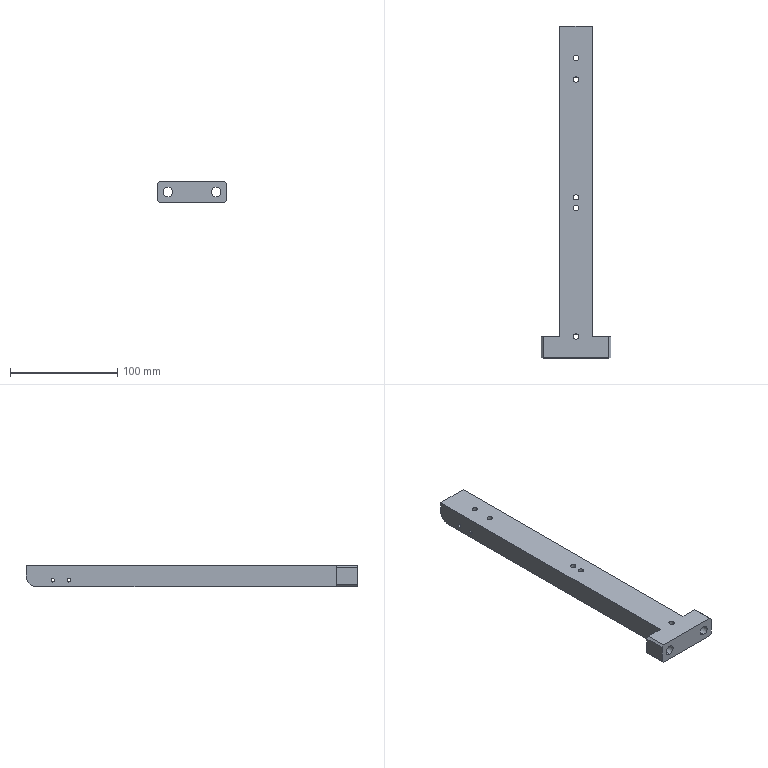Part | SolidWorks | features HoleWzd 3, Chamfer 1, Extrusion 1, Fillet 1 | 1 solid | 33 faces | box 65 x 310 x 20 mm | volume 194175 mm3 | cylinder 19 | plane 14 | commonest cylinder face diameters 5 x10 3.3 x4 9 x4 20 x1
STEP:
#1=CARTESIAN_POINT('',(15.,285.,4.35));
#2=VERTEX_POINT('',#1);
#3=CARTESIAN_POINT('',(15.,285.,7.65));
#4=VERTEX_POINT('',#3);
#5=CARTESIAN_POINT('',(15.,285.,6.));
#6=DIRECTION('',(-1.,0.,0.));
#7=DIRECTION('',(0.,-1.,0.));
#8=AXIS2_PLACEMENT_3D('',#5,#6,#7);
#9=CIRCLE('',#8,1.65);
#10=EDGE_CURVE('',#2,#4,#9,.T.);
#11=ORIENTED_EDGE('',*,*,#10,.F.);
#12=CARTESIAN_POINT('',(-15.,285.,4.35));
#13=VERTEX_POINT('',#12);
#14=CARTESIAN_POINT('',(-15.,285.,4.35));
#15=DIRECTION('',(-1.,0.,0.));
#16=VECTOR('',#15,1000.);
#17=LINE('',#14,#16);
#18=EDGE_CURVE('',#2,#13,#17,.T.);
#19=ORIENTED_EDGE('',*,*,#18,.T.);
#20=CARTESIAN_POINT('',(-15.,285.,7.65));
#21=VERTEX_POINT('',#20);
#22=CARTESIAN_POINT('',(-15.,285.,6.));
#23=DIRECTION('',(-1.,0.,0.));
#24=DIRECTION('',(0.,0.,1.));
#25=AXIS2_PLACEMENT_3D('',#22,#23,#24);
#26=CIRCLE('',#25,1.65);
#27=EDGE_CURVE('',#13,#21,#26,.T.);
#28=ORIENTED_EDGE('',*,*,#27,.T.);
#29=CARTESIAN_POINT('',(-15.,285.,7.65));
#30=DIRECTION('',(-1.,0.,0.));
#31=VECTOR('',#30,1000.);
#32=LINE('',#29,#31);
#33=EDGE_CURVE('',#4,#21,#32,.T.);
#34=ORIENTED_EDGE('',*,*,#33,.F.);
#35=EDGE_LOOP('',(#11,#19,#28,#34));
#36=FACE_OUTER_BOUND('',#35,.T.);
#37=CARTESIAN_POINT('',(-15.,285.,6.));
#38=DIRECTION('',(-1.,0.,0.));
#39=DIRECTION('',(0.,0.,1.));
#40=AXIS2_PLACEMENT_3D('',#37,#38,#39);
#41=CYLINDRICAL_SURFACE('',#40,1.65);
#42=ADVANCED_FACE('',(#36),#41,.F.);
#43=CARTESIAN_POINT('',(15.,270.,4.35));
#44=VERTEX_POINT('',#43);
#45=CARTESIAN_POINT('',(15.,270.,7.65));
#46=VERTEX_POINT('',#45);
#47=CARTESIAN_POINT('',(15.,270.,6.));
#48=DIRECTION('',(-1.,0.,0.));
#49=DIRECTION('',(0.,-1.,0.));
#50=AXIS2_PLACEMENT_3D('',#47,#48,#49);
#51=CIRCLE('',#50,1.65);
#52=EDGE_CURVE('',#44,#46,#51,.T.);
#53=ORIENTED_EDGE('',*,*,#52,.F.);
#54=CARTESIAN_POINT('',(-15.,270.,4.35));
#55=VERTEX_POINT('',#54);
#56=CARTESIAN_POINT('',(-15.,270.,4.35));
#57=DIRECTION('',(-1.,0.,0.));
#58=VECTOR('',#57,1000.);
#59=LINE('',#56,#58);
#60=EDGE_CURVE('',#44,#55,#59,.T.);
#61=ORIENTED_EDGE('',*,*,#60,.T.);
#62=CARTESIAN_POINT('',(-15.,270.,7.65));
#63=VERTEX_POINT('',#62);
#64=CARTESIAN_POINT('',(-15.,270.,6.));
#65=DIRECTION('',(-1.,0.,0.));
#66=DIRECTION('',(0.,0.,1.));
#67=AXIS2_PLACEMENT_3D('',#64,#65,#66);
#68=CIRCLE('',#67,1.65);
#69=EDGE_CURVE('',#55,#63,#68,.T.);
#70=ORIENTED_EDGE('',*,*,#69,.T.);
#71=CARTESIAN_POINT('',(-15.,270.,7.65));
#72=DIRECTION('',(-1.,0.,0.));
#73=VECTOR('',#72,1000.);
#74=LINE('',#71,#73);
#75=EDGE_CURVE('',#46,#63,#74,.T.);
#76=ORIENTED_EDGE('',*,*,#75,.F.);
#77=EDGE_LOOP('',(#53,#61,#70,#76));
#78=FACE_OUTER_BOUND('',#77,.T.);
#79=CARTESIAN_POINT('',(-15.,270.,6.));
#80=DIRECTION('',(-1.,0.,0.));
#81=DIRECTION('',(0.,0.,1.));
#82=AXIS2_PLACEMENT_3D('',#79,#80,#81);
#83=CYLINDRICAL_SURFACE('',#82,1.65);
#84=ADVANCED_FACE('',(#78),#83,.F.);
#85=CARTESIAN_POINT('',(-2.5,280.,0.));
#86=VERTEX_POINT('',#85);
#87=CARTESIAN_POINT('',(2.5,280.,0.));
#88=VERTEX_POINT('',#87);
#89=CARTESIAN_POINT('',(0.,280.,0.));
#90=DIRECTION('',(0.,0.,1.));
#91=DIRECTION('',(1.,0.,0.));
#92=AXIS2_PLACEMENT_3D('',#89,#90,#91);
#93=CIRCLE('',#92,2.5);
#94=EDGE_CURVE('',#86,#88,#93,.T.);
#95=ORIENTED_EDGE('',*,*,#94,.F.);
#96=CARTESIAN_POINT('',(-2.5,280.,20.));
#97=VERTEX_POINT('',#96);
#98=CARTESIAN_POINT('',(-2.5,280.,20.));
#99=DIRECTION('',(0.,0.,1.));
#100=VECTOR('',#99,1000.);
#101=LINE('',#98,#100);
#102=EDGE_CURVE('',#86,#97,#101,.T.);
#103=ORIENTED_EDGE('',*,*,#102,.T.);
#104=CARTESIAN_POINT('',(2.5,280.,20.));
#105=VERTEX_POINT('',#104);
#106=CARTESIAN_POINT('',(0.,280.,20.));
#107=DIRECTION('',(0.,0.,1.));
#108=DIRECTION('',(1.,0.,0.));
#109=AXIS2_PLACEMENT_3D('',#106,#107,#108);
#110=CIRCLE('',#109,2.5);
#111=EDGE_CURVE('',#97,#105,#110,.T.);
#112=ORIENTED_EDGE('',*,*,#111,.T.);
#113=CARTESIAN_POINT('',(2.5,280.,20.));
#114=DIRECTION('',(0.,0.,1.));
#115=VECTOR('',#114,1000.);
#116=LINE('',#113,#115);
#117=EDGE_CURVE('',#88,#105,#116,.T.);
#118=ORIENTED_EDGE('',*,*,#117,.F.);
#119=EDGE_LOOP('',(#95,#103,#112,#118));
#120=FACE_OUTER_BOUND('',#119,.T.);
#121=CARTESIAN_POINT('',(0.,280.,20.));
#122=DIRECTION('',(0.,0.,1.));
#123=DIRECTION('',(1.,0.,0.));
#124=AXIS2_PLACEMENT_3D('',#121,#122,#123);
#125=CYLINDRICAL_SURFACE('',#124,2.5);
#126=ADVANCED_FACE('',(#120),#125,.F.);
#127=CARTESIAN_POINT('',(-2.5,150.,0.));
#128=VERTEX_POINT('',#127);
#129=CARTESIAN_POINT('',(2.5,150.,0.));
#130=VERTEX_POINT('',#129);
#131=CARTESIAN_POINT('',(0.,150.,0.));
#132=DIRECTION('',(0.,0.,1.));
#133=DIRECTION('',(1.,0.,0.));
#134=AXIS2_PLACEMENT_3D('',#131,#132,#133);
#135=CIRCLE('',#134,2.5);
#136=EDGE_CURVE('',#128,#130,#135,.T.);
#137=ORIENTED_EDGE('',*,*,#136,.F.);
#138=CARTESIAN_POINT('',(-2.5,150.,20.));
#139=VERTEX_POINT('',#138);
#140=CARTESIAN_POINT('',(-2.5,150.,20.));
#141=DIRECTION('',(0.,0.,1.));
#142=VECTOR('',#141,1000.);
#143=LINE('',#140,#142);
#144=EDGE_CURVE('',#128,#139,#143,.T.);
#145=ORIENTED_EDGE('',*,*,#144,.T.);
#146=CARTESIAN_POINT('',(2.5,150.,20.));
#147=VERTEX_POINT('',#146);
#148=CARTESIAN_POINT('',(0.,150.,20.));
#149=DIRECTION('',(0.,0.,1.));
#150=DIRECTION('',(1.,0.,0.));
#151=AXIS2_PLACEMENT_3D('',#148,#149,#150);
#152=CIRCLE('',#151,2.5);
#153=EDGE_CURVE('',#139,#147,#152,.T.);
#154=ORIENTED_EDGE('',*,*,#153,.T.);
#155=CARTESIAN_POINT('',(2.5,150.,20.));
#156=DIRECTION('',(0.,0.,1.));
#157=VECTOR('',#156,1000.);
#158=LINE('',#155,#157);
#159=EDGE_CURVE('',#130,#147,#158,.T.);
#160=ORIENTED_EDGE('',*,*,#159,.F.);
#161=EDGE_LOOP('',(#137,#145,#154,#160));
#162=FACE_OUTER_BOUND('',#161,.T.);
#163=CARTESIAN_POINT('',(0.,150.,20.));
#164=DIRECTION('',(0.,0.,1.));
#165=DIRECTION('',(1.,0.,0.));
#166=AXIS2_PLACEMENT_3D('',#163,#164,#165);
#167=CYLINDRICAL_SURFACE('',#166,2.5);
#168=ADVANCED_FACE('',(#162),#167,.F.);
#169=CARTESIAN_POINT('',(-2.5,20.,0.));
#170=VERTEX_POINT('',#169);
#171=CARTESIAN_POINT('',(2.5,20.,0.));
#172=VERTEX_POINT('',#171);
#173=CARTESIAN_POINT('',(0.,20.,0.));
#174=DIRECTION('',(0.,0.,1.));
#175=DIRECTION('',(1.,0.,0.));
#176=AXIS2_PLACEMENT_3D('',#173,#174,#175);
#177=CIRCLE('',#176,2.5);
#178=EDGE_CURVE('',#170,#172,#177,.T.);
#179=ORIENTED_EDGE('',*,*,#178,.F.);
#180=CARTESIAN_POINT('',(-2.5,20.,20.));
#181=VERTEX_POINT('',#180);
#182=CARTESIAN_POINT('',(-2.5,20.,20.));
#183=DIRECTION('',(0.,0.,1.));
#184=VECTOR('',#183,1000.);
#185=LINE('',#182,#184);
#186=EDGE_CURVE('',#170,#181,#185,.T.);
#187=ORIENTED_EDGE('',*,*,#186,.T.);
#188=CARTESIAN_POINT('',(2.5,20.,20.));
#189=VERTEX_POINT('',#188);
#190=CARTESIAN_POINT('',(0.,20.,20.));
#191=DIRECTION('',(0.,0.,1.));
#192=DIRECTION('',(1.,0.,0.));
#193=AXIS2_PLACEMENT_3D('',#190,#191,#192);
#194=CIRCLE('',#193,2.5);
#195=EDGE_CURVE('',#181,#189,#194,.T.);
#196=ORIENTED_EDGE('',*,*,#195,.T.);
#197=CARTESIAN_POINT('',(2.5,20.,20.));
#198=DIRECTION('',(0.,0.,1.));
#199=VECTOR('',#198,1000.);
#200=LINE('',#197,#199);
#201=EDGE_CURVE('',#172,#189,#200,.T.);
#202=ORIENTED_EDGE('',*,*,#201,.F.);
#203=EDGE_LOOP('',(#179,#187,#196,#202));
#204=FACE_OUTER_BOUND('',#203,.T.);
#205=CARTESIAN_POINT('',(0.,20.,20.));
#206=DIRECTION('',(0.,0.,1.));
#207=DIRECTION('',(1.,0.,0.));
#208=AXIS2_PLACEMENT_3D('',#205,#206,#207);
#209=CYLINDRICAL_SURFACE('',#208,2.5);
#210=ADVANCED_FACE('',(#204),#209,.F.);
#211=CARTESIAN_POINT('',(-2.5,260.,0.));
#212=VERTEX_POINT('',#211);
#213=CARTESIAN_POINT('',(2.5,260.,0.));
#214=VERTEX_POINT('',#213);
#215=CARTESIAN_POINT('',(0.,260.,0.));
#216=DIRECTION('',(0.,0.,1.));
#217=DIRECTION('',(1.,0.,0.));
#218=AXIS2_PLACEMENT_3D('',#215,#216,#217);
#219=CIRCLE('',#218,2.5);
#220=EDGE_CURVE('',#212,#214,#219,.T.);
#221=ORIENTED_EDGE('',*,*,#220,.F.);
#222=CARTESIAN_POINT('',(-2.5,260.,20.));
#223=VERTEX_POINT('',#222);
#224=CARTESIAN_POINT('',(-2.5,260.,20.));
#225=DIRECTION('',(0.,0.,1.));
#226=VECTOR('',#225,1000.);
#227=LINE('',#224,#226);
#228=EDGE_CURVE('',#212,#223,#227,.T.);
#229=ORIENTED_EDGE('',*,*,#228,.T.);
#230=CARTESIAN_POINT('',(2.5,260.,20.));
#231=VERTEX_POINT('',#230);
#232=CARTESIAN_POINT('',(0.,260.,20.));
#233=DIRECTION('',(0.,0.,1.));
#234=DIRECTION('',(1.,0.,0.));
#235=AXIS2_PLACEMENT_3D('',#232,#233,#234);
#236=CIRCLE('',#235,2.5);
#237=EDGE_CURVE('',#223,#231,#236,.T.);
#238=ORIENTED_EDGE('',*,*,#237,.T.);
#239=CARTESIAN_POINT('',(2.5,260.,20.));
#240=DIRECTION('',(0.,0.,1.));
#241=VECTOR('',#240,1000.);
#242=LINE('',#239,#241);
#243=EDGE_CURVE('',#214,#231,#242,.T.);
#244=ORIENTED_EDGE('',*,*,#243,.F.);
#245=EDGE_LOOP('',(#221,#229,#238,#244));
#246=FACE_OUTER_BOUND('',#245,.T.);
#247=CARTESIAN_POINT('',(0.,260.,20.));
#248=DIRECTION('',(0.,0.,1.));
#249=DIRECTION('',(1.,0.,0.));
#250=AXIS2_PLACEMENT_3D('',#247,#248,#249);
#251=CYLINDRICAL_SURFACE('',#250,2.5);
#252=ADVANCED_FACE('',(#246),#251,.F.);
#253=CARTESIAN_POINT('',(-2.5,140.,0.));
#254=VERTEX_POINT('',#253);
#255=CARTESIAN_POINT('',(2.5,140.,0.));
#256=VERTEX_POINT('',#255);
#257=CARTESIAN_POINT('',(0.,140.,0.));
#258=DIRECTION('',(0.,0.,1.));
#259=DIRECTION('',(1.,0.,0.));
#260=AXIS2_PLACEMENT_3D('',#257,#258,#259);
#261=CIRCLE('',#260,2.5);
#262=EDGE_CURVE('',#254,#256,#261,.T.);
#263=ORIENTED_EDGE('',*,*,#262,.F.);
#264=CARTESIAN_POINT('',(-2.5,140.,20.));
#265=VERTEX_POINT('',#264);
#266=CARTESIAN_POINT('',(-2.5,140.,20.));
#267=DIRECTION('',(0.,0.,1.));
#268=VECTOR('',#267,1000.);
#269=LINE('',#266,#268);
#270=EDGE_CURVE('',#254,#265,#269,.T.);
#271=ORIENTED_EDGE('',*,*,#270,.T.);
#272=CARTESIAN_POINT('',(2.5,140.,20.));
#273=VERTEX_POINT('',#272);
#274=CARTESIAN_POINT('',(0.,140.,20.));
#275=DIRECTION('',(0.,0.,1.));
#276=DIRECTION('',(1.,0.,0.));
#277=AXIS2_PLACEMENT_3D('',#274,#275,#276);
#278=CIRCLE('',#277,2.5);
#279=EDGE_CURVE('',#265,#273,#278,.T.);
#280=ORIENTED_EDGE('',*,*,#279,.T.);
#281=CARTESIAN_POINT('',(2.5,140.,20.));
#282=DIRECTION('',(0.,0.,1.));
#283=VECTOR('',#282,1000.);
#284=LINE('',#281,#283);
#285=EDGE_CURVE('',#256,#273,#284,.T.);
#286=ORIENTED_EDGE('',*,*,#285,.F.);
#287=EDGE_LOOP('',(#263,#271,#280,#286));
#288=FACE_OUTER_BOUND('',#287,.T.);
#289=CARTESIAN_POINT('',(0.,140.,20.));
#290=DIRECTION('',(0.,0.,1.));
#291=DIRECTION('',(1.,0.,0.));
#292=AXIS2_PLACEMENT_3D('',#289,#290,#291);
#293=CYLINDRICAL_SURFACE('',#292,2.5);
#294=ADVANCED_FACE('',(#288),#293,.F.);
#295=CARTESIAN_POINT('',(22.5,0.,5.5));
#296=VERTEX_POINT('',#295);
#297=CARTESIAN_POINT('',(22.5,0.,14.5));
#298=VERTEX_POINT('',#297);
#299=CARTESIAN_POINT('',(22.5,0.,10.));
#300=DIRECTION('',(0.,1.,0.));
#301=DIRECTION('',(0.,0.,1.));
#302=AXIS2_PLACEMENT_3D('',#299,#300,#301);
#303=CIRCLE('',#302,4.5);
#304=EDGE_CURVE('',#296,#298,#303,.T.);
#305=ORIENTED_EDGE('',*,*,#304,.F.);
#306=CARTESIAN_POINT('',(22.5,20.,5.5));
#307=VERTEX_POINT('',#306);
#308=CARTESIAN_POINT('',(22.5,20.,5.5));
#309=DIRECTION('',(0.,1.,0.));
#310=VECTOR('',#309,1000.);
#311=LINE('',#308,#310);
#312=EDGE_CURVE('',#296,#307,#311,.T.);
#313=ORIENTED_EDGE('',*,*,#312,.T.);
#314=CARTESIAN_POINT('',(22.5,20.,14.5));
#315=VERTEX_POINT('',#314);
#316=CARTESIAN_POINT('',(22.5,20.,10.));
#317=DIRECTION('',(0.,1.,0.));
#318=DIRECTION('',(0.,0.,1.));
#319=AXIS2_PLACEMENT_3D('',#316,#317,#318);
#320=CIRCLE('',#319,4.5);
#321=EDGE_CURVE('',#307,#315,#320,.T.);
#322=ORIENTED_EDGE('',*,*,#321,.T.);
#323=CARTESIAN_POINT('',(22.5,20.,14.5));
#324=DIRECTION('',(0.,1.,0.));
#325=VECTOR('',#324,1000.);
#326=LINE('',#323,#325);
#327=EDGE_CURVE('',#298,#315,#326,.T.);
#328=ORIENTED_EDGE('',*,*,#327,.F.);
#329=EDGE_LOOP('',(#305,#313,#322,#328));
#330=FACE_OUTER_BOUND('',#329,.T.);
#331=CARTESIAN_POINT('',(22.5,20.,10.));
#332=DIRECTION('',(0.,1.,0.));
#333=DIRECTION('',(0.,0.,1.));
#334=AXIS2_PLACEMENT_3D('',#331,#332,#333);
#335=CYLINDRICAL_SURFACE('',#334,4.5);
#336=ADVANCED_FACE('',(#330),#335,.F.);
#337=CARTESIAN_POINT('',(-22.5,0.,5.5));
#338=VERTEX_POINT('',#337);
#339=CARTESIAN_POINT('',(-22.5,0.,14.5));
#340=VERTEX_POINT('',#339);
#341=CARTESIAN_POINT('',(-22.5,0.,10.));
#342=DIRECTION('',(0.,1.,0.));
#343=DIRECTION('',(0.,0.,1.));
#344=AXIS2_PLACEMENT_3D('',#341,#342,#343);
#345=CIRCLE('',#344,4.5);
#346=EDGE_CURVE('',#338,#340,#345,.T.);
#347=ORIENTED_EDGE('',*,*,#346,.F.);
#348=CARTESIAN_POINT('',(-22.5,20.,5.5));
#349=VERTEX_POINT('',#348);
#350=CARTESIAN_POINT('',(-22.5,20.,5.5));
#351=DIRECTION('',(0.,1.,0.));
#352=VECTOR('',#351,1000.);
#353=LINE('',#350,#352);
#354=EDGE_CURVE('',#338,#349,#353,.T.);
#355=ORIENTED_EDGE('',*,*,#354,.T.);
#356=CARTESIAN_POINT('',(-22.5,20.,14.5));
#357=VERTEX_POINT('',#356);
#358=CARTESIAN_POINT('',(-22.5,20.,10.));
#359=DIRECTION('',(0.,1.,0.));
#360=DIRECTION('',(0.,0.,1.));
#361=AXIS2_PLACEMENT_3D('',#358,#359,#360);
#362=CIRCLE('',#361,4.5);
#363=EDGE_CURVE('',#349,#357,#362,.T.);
#364=ORIENTED_EDGE('',*,*,#363,.T.);
#365=CARTESIAN_POINT('',(-22.5,20.,14.5));
#366=DIRECTION('',(0.,1.,0.));
#367=VECTOR('',#366,1000.);
#368=LINE('',#365,#367);
#369=EDGE_CURVE('',#340,#357,#368,.T.);
#370=ORIENTED_EDGE('',*,*,#369,.F.);
#371=EDGE_LOOP('',(#347,#355,#364,#370));
#372=FACE_OUTER_BOUND('',#371,.T.);
#373=CARTESIAN_POINT('',(-22.5,20.,10.));
#374=DIRECTION('',(0.,1.,0.));
#375=DIRECTION('',(0.,0.,1.));
#376=AXIS2_PLACEMENT_3D('',#373,#374,#375);
#377=CYLINDRICAL_SURFACE('',#376,4.5);
#378=ADVANCED_FACE('',(#372),#377,.F.);
#379=CARTESIAN_POINT('',(-15.,285.,6.));
#380=DIRECTION('',(-1.,0.,0.));
#381=DIRECTION('',(0.,0.,1.));
#382=AXIS2_PLACEMENT_3D('',#379,#380,#381);
#383=CIRCLE('',#382,1.65);
#384=EDGE_CURVE('',#21,#13,#383,.T.);
#385=ORIENTED_EDGE('',*,*,#384,.F.);
#386=ORIENTED_EDGE('',*,*,#27,.F.);
#387=EDGE_LOOP('',(#385,#386));
#388=FACE_BOUND('',#387,.T.);
#389=CARTESIAN_POINT('',(-15.,270.,6.));
#390=DIRECTION('',(-1.,0.,0.));
#391=DIRECTION('',(0.,0.,1.));
#392=AXIS2_PLACEMENT_3D('',#389,#390,#391);
#393=CIRCLE('',#392,1.65);
#394=EDGE_CURVE('',#63,#55,#393,.T.);
#395=ORIENTED_EDGE('',*,*,#394,.F.);
#396=ORIENTED_EDGE('',*,*,#69,.F.);
#397=EDGE_LOOP('',(#395,#396));
#398=FACE_BOUND('',#397,.T.);
#399=CARTESIAN_POINT('',(-15.,310.,20.));
#400=VERTEX_POINT('',#399);
#401=CARTESIAN_POINT('',(-15.,310.,10.));
#402=VERTEX_POINT('',#401);
#403=CARTESIAN_POINT('',(-15.,310.,20.));
#404=DIRECTION('',(0.,0.,-1.));
#405=VECTOR('',#404,1000.);
#406=LINE('',#403,#405);
#407=EDGE_CURVE('',#400,#402,#406,.T.);
#408=ORIENTED_EDGE('',*,*,#407,.T.);
#409=CARTESIAN_POINT('',(-15.,300.,0.));
#410=VERTEX_POINT('',#409);
#411=CARTESIAN_POINT('',(-15.,300.,10.));
#412=DIRECTION('',(-1.,0.,0.));
#413=DIRECTION('',(0.,1.,0.));
#414=AXIS2_PLACEMENT_3D('',#411,#412,#413);
#415=CIRCLE('',#414,10.);
#416=EDGE_CURVE('',#402,#410,#415,.T.);
#417=ORIENTED_EDGE('',*,*,#416,.T.);
#418=CARTESIAN_POINT('',(-15.,20.,0.));
#419=VERTEX_POINT('',#418);
#420=CARTESIAN_POINT('',(-15.,310.,0.));
#421=DIRECTION('',(0.,-1.,0.));
#422=VECTOR('',#421,1000.);
#423=LINE('',#420,#422);
#424=EDGE_CURVE('',#410,#419,#423,.T.);
#425=ORIENTED_EDGE('',*,*,#424,.T.);
#426=CARTESIAN_POINT('',(-15.,20.,20.));
#427=VERTEX_POINT('',#426);
#428=CARTESIAN_POINT('',(-15.,20.,20.));
#429=DIRECTION('',(0.,0.,-1.));
#430=VECTOR('',#429,1000.);
#431=LINE('',#428,#430);
#432=EDGE_CURVE('',#427,#419,#431,.T.);
#433=ORIENTED_EDGE('',*,*,#432,.F.);
#434=CARTESIAN_POINT('',(-15.,310.,20.));
#435=DIRECTION('',(0.,-1.,0.));
#436=VECTOR('',#435,1000.);
#437=LINE('',#434,#436);
#438=EDGE_CURVE('',#400,#427,#437,.T.);
#439=ORIENTED_EDGE('',*,*,#438,.F.);
#440=EDGE_LOOP('',(#408,#417,#425,#433,#439));
#441=FACE_OUTER_BOUND('',#440,.T.);
#442=CARTESIAN_POINT('',(-15.,310.,20.));
#443=DIRECTION('',(1.,0.,0.));
#444=DIRECTION('',(0.,1.,0.));
#445=AXIS2_PLACEMENT_3D('',#442,#443,#444);
#446=PLANE('',#445);
#447=ADVANCED_FACE('',(#388,#398,#441),#446,.F.);
#448=CARTESIAN_POINT('',(-22.5,20.,10.));
#449=DIRECTION('',(0.,1.,0.));
#450=DIRECTION('',(0.,0.,1.));
#451=AXIS2_PLACEMENT_3D('',#448,#449,#450);
#452=CIRCLE('',#451,4.5);
#453=EDGE_CURVE('',#357,#349,#452,.T.);
#454=ORIENTED_EDGE('',*,*,#453,.F.);
#455=ORIENTED_EDGE('',*,*,#363,.F.);
#456=EDGE_LOOP('',(#454,#455));
#457=FACE_BOUND('',#456,.T.);
#458=CARTESIAN_POINT('',(-32.5,20.,18.));
#459=VERTEX_POINT('',#458);
#460=CARTESIAN_POINT('',(-32.5,20.,2.));
#461=VERTEX_POINT('',#460);
#462=CARTESIAN_POINT('',(-32.5,20.,20.));
#463=DIRECTION('',(0.,0.,-1.));
#464=VECTOR('',#463,1000.);
#465=LINE('',#462,#464);
#466=EDGE_CURVE('',#459,#461,#465,.T.);
#467=ORIENTED_EDGE('',*,*,#466,.F.);
#468=CARTESIAN_POINT('',(-30.5,20.,20.));
#469=VERTEX_POINT('',#468);
#470=CARTESIAN_POINT('',(-30.5,20.,20.));
#471=DIRECTION('',(0.7071,0.,0.7071));
#472=VECTOR('',#471,1000.);
#473=LINE('',#470,#472);
#474=EDGE_CURVE('',#459,#469,#473,.T.);
#475=ORIENTED_EDGE('',*,*,#474,.T.);
#476=CARTESIAN_POINT('',(-15.,20.,20.));
#477=DIRECTION('',(-1.,0.,0.));
#478=VECTOR('',#477,1000.);
#479=LINE('',#476,#478);
#480=EDGE_CURVE('',#427,#469,#479,.T.);
#481=ORIENTED_EDGE('',*,*,#480,.F.);
#482=ORIENTED_EDGE('',*,*,#432,.T.);
#483=CARTESIAN_POINT('',(-30.5,20.,0.));
#484=VERTEX_POINT('',#483);
#485=CARTESIAN_POINT('',(-15.,20.,0.));
#486=DIRECTION('',(-1.,0.,0.));
#487=VECTOR('',#486,1000.);
#488=LINE('',#485,#487);
#489=EDGE_CURVE('',#419,#484,#488,.T.);
#490=ORIENTED_EDGE('',*,*,#489,.T.);
#491=CARTESIAN_POINT('',(-32.5,20.,2.));
#492=DIRECTION('',(-0.7071,0.,0.7071));
#493=VECTOR('',#492,1000.);
#494=LINE('',#491,#493);
#495=EDGE_CURVE('',#484,#461,#494,.T.);
#496=ORIENTED_EDGE('',*,*,#495,.T.);
#497=EDGE_LOOP('',(#467,#475,#481,#482,#490,#496));
#498=FACE_OUTER_BOUND('',#497,.T.);
#499=CARTESIAN_POINT('',(-15.,20.,20.));
#500=DIRECTION('',(0.,-1.,0.));
#501=DIRECTION('',(1.,0.,0.));
#502=AXIS2_PLACEMENT_3D('',#499,#500,#501);
#503=PLANE('',#502);
#504=ADVANCED_FACE('',(#457,#498),#503,.F.);
#505=CARTESIAN_POINT('',(-32.5,0.,18.));
#506=VERTEX_POINT('',#505);
#507=CARTESIAN_POINT('',(-32.5,0.,2.));
#508=VERTEX_POINT('',#507);
#509=CARTESIAN_POINT('',(-32.5,0.,20.));
#510=DIRECTION('',(0.,0.,-1.));
#511=VECTOR('',#510,1000.);
#512=LINE('',#509,#511);
#513=EDGE_CURVE('',#506,#508,#512,.T.);
#514=ORIENTED_EDGE('',*,*,#513,.F.);
#515=CARTESIAN_POINT('',(-32.5,20.,18.));
#516=DIRECTION('',(0.,1.,0.));
#517=VECTOR('',#516,1000.);
#518=LINE('',#515,#517);
#519=EDGE_CURVE('',#506,#459,#518,.T.);
#520=ORIENTED_EDGE('',*,*,#519,.T.);
#521=ORIENTED_EDGE('',*,*,#466,.T.);
#522=CARTESIAN_POINT('',(-32.5,0.,2.));
#523=DIRECTION('',(0.,-1.,0.));
#524=VECTOR('',#523,1000.);
#525=LINE('',#522,#524);
#526=EDGE_CURVE('',#461,#508,#525,.T.);
#527=ORIENTED_EDGE('',*,*,#526,.T.);
#528=EDGE_LOOP('',(#514,#520,#521,#527));
#529=FACE_OUTER_BOUND('',#528,.T.);
#530=CARTESIAN_POINT('',(-32.5,20.,20.));
#531=DIRECTION('',(1.,0.,0.));
#532=DIRECTION('',(0.,1.,0.));
#533=AXIS2_PLACEMENT_3D('',#530,#531,#532);
#534=PLANE('',#533);
#535=ADVANCED_FACE('',(#529),#534,.F.);
#536=CARTESIAN_POINT('',(22.5,0.,10.));
#537=DIRECTION('',(0.,1.,0.));
#538=DIRECTION('',(0.,0.,1.));
#539=AXIS2_PLACEMENT_3D('',#536,#537,#538);
#540=CIRCLE('',#539,4.5);
#541=EDGE_CURVE('',#298,#296,#540,.T.);
#542=ORIENTED_EDGE('',*,*,#541,.T.);
#543=ORIENTED_EDGE('',*,*,#304,.T.);
#544=EDGE_LOOP('',(#542,#543));
#545=FACE_BOUND('',#544,.T.);
#546=CARTESIAN_POINT('',(-22.5,0.,10.));
#547=DIRECTION('',(0.,1.,0.));
#548=DIRECTION('',(0.,0.,1.));
#549=AXIS2_PLACEMENT_3D('',#546,#547,#548);
#550=CIRCLE('',#549,4.5);
#551=EDGE_CURVE('',#340,#338,#550,.T.);
#552=ORIENTED_EDGE('',*,*,#551,.T.);
#553=ORIENTED_EDGE('',*,*,#346,.T.);
#554=EDGE_LOOP('',(#552,#553));
#555=FACE_BOUND('',#554,.T.);
#556=CARTESIAN_POINT('',(32.5,0.,18.));
#557=VERTEX_POINT('',#556);
#558=CARTESIAN_POINT('',(32.5,0.,2.));
#559=VERTEX_POINT('',#558);
#560=CARTESIAN_POINT('',(32.5,0.,20.));
#561=DIRECTION('',(0.,0.,-1.));
#562=VECTOR('',#561,1000.);
#563=LINE('',#560,#562);
#564=EDGE_CURVE('',#557,#559,#563,.T.);
#565=ORIENTED_EDGE('',*,*,#564,.F.);
#566=CARTESIAN_POINT('',(30.5,0.,20.));
#567=VERTEX_POINT('',#566);
#568=CARTESIAN_POINT('',(30.5,0.,20.));
#569=DIRECTION('',(-0.7071,0.,0.7071));
#570=VECTOR('',#569,1000.);
#571=LINE('',#568,#570);
#572=EDGE_CURVE('',#557,#567,#571,.T.);
#573=ORIENTED_EDGE('',*,*,#572,.T.);
#574=CARTESIAN_POINT('',(-30.5,0.,20.));
#575=VERTEX_POINT('',#574);
#576=CARTESIAN_POINT('',(-32.5,0.,20.));
#577=DIRECTION('',(1.,0.,0.));
#578=VECTOR('',#577,1000.);
#579=LINE('',#576,#578);
#580=EDGE_CURVE('',#575,#567,#579,.T.);
#581=ORIENTED_EDGE('',*,*,#580,.F.);
#582=CARTESIAN_POINT('',(-30.5,0.,20.));
#583=DIRECTION('',(-0.7071,0.,-0.7071));
#584=VECTOR('',#583,1000.);
#585=LINE('',#582,#584);
#586=EDGE_CURVE('',#575,#506,#585,.T.);
#587=ORIENTED_EDGE('',*,*,#586,.T.);
#588=ORIENTED_EDGE('',*,*,#513,.T.);
#589=CARTESIAN_POINT('',(-30.5,0.,0.));
#590=VERTEX_POINT('',#589);
#591=CARTESIAN_POINT('',(-32.5,0.,2.));
#592=DIRECTION('',(0.7071,0.,-0.7071));
#593=VECTOR('',#592,1000.);
#594=LINE('',#591,#593);
#595=EDGE_CURVE('',#508,#590,#594,.T.);
#596=ORIENTED_EDGE('',*,*,#595,.T.);
#597=CARTESIAN_POINT('',(30.5,0.,0.));
#598=VERTEX_POINT('',#597);
#599=CARTESIAN_POINT('',(-32.5,0.,0.));
#600=DIRECTION('',(1.,0.,0.));
#601=VECTOR('',#600,1000.);
#602=LINE('',#599,#601);
#603=EDGE_CURVE('',#590,#598,#602,.T.);
#604=ORIENTED_EDGE('',*,*,#603,.T.);
#605=CARTESIAN_POINT('',(32.5,0.,2.));
#606=DIRECTION('',(0.7071,0.,0.7071));
#607=VECTOR('',#606,1000.);
#608=LINE('',#605,#607);
#609=EDGE_CURVE('',#598,#559,#608,.T.);
#610=ORIENTED_EDGE('',*,*,#609,.T.);
#611=EDGE_LOOP('',(#565,#573,#581,#587,#588,#596,#604,#610));
#612=FACE_OUTER_BOUND('',#611,.T.);
#613=CARTESIAN_POINT('',(-32.5,0.,20.));
#614=DIRECTION('',(0.,1.,0.));
#615=DIRECTION('',(0.,0.,1.));
#616=AXIS2_PLACEMENT_3D('',#613,#614,#615);
#617=PLANE('',#616);
#618=ADVANCED_FACE('',(#545,#555,#612),#617,.F.);
#619=CARTESIAN_POINT('',(32.5,20.,18.));
#620=VERTEX_POINT('',#619);
#621=CARTESIAN_POINT('',(32.5,20.,2.));
#622=VERTEX_POINT('',#621);
#623=CARTESIAN_POINT('',(32.5,20.,20.));
#624=DIRECTION('',(0.,0.,-1.));
#625=VECTOR('',#624,1000.);
#626=LINE('',#623,#625);
#627=EDGE_CURVE('',#620,#622,#626,.T.);
#628=ORIENTED_EDGE('',*,*,#627,.F.);
#629=CARTESIAN_POINT('',(32.5,20.,18.));
#630=DIRECTION('',(0.,-1.,0.));
#631=VECTOR('',#630,1000.);
#632=LINE('',#629,#631);
#633=EDGE_CURVE('',#620,#557,#632,.T.);
#634=ORIENTED_EDGE('',*,*,#633,.T.);
#635=ORIENTED_EDGE('',*,*,#564,.T.);
#636=CARTESIAN_POINT('',(32.5,20.,2.));
#637=DIRECTION('',(0.,1.,0.));
#638=VECTOR('',#637,1000.);
#639=LINE('',#636,#638);
#640=EDGE_CURVE('',#559,#622,#639,.T.);
#641=ORIENTED_EDGE('',*,*,#640,.T.);
#642=EDGE_LOOP('',(#628,#634,#635,#641));
#643=FACE_OUTER_BOUND('',#642,.T.);
#644=CARTESIAN_POINT('',(32.5,20.,20.));
#645=DIRECTION('',(-1.,0.,0.));
#646=DIRECTION('',(0.,-1.,0.));
#647=AXIS2_PLACEMENT_3D('',#644,#645,#646);
#648=PLANE('',#647);
#649=ADVANCED_FACE('',(#643),#648,.F.);
#650=CARTESIAN_POINT('',(22.5,20.,10.));
#651=DIRECTION('',(0.,1.,0.));
#652=DIRECTION('',(0.,0.,1.));
#653=AXIS2_PLACEMENT_3D('',#650,#651,#652);
#654=CIRCLE('',#653,4.5);
#655=EDGE_CURVE('',#315,#307,#654,.T.);
#656=ORIENTED_EDGE('',*,*,#655,.F.);
#657=ORIENTED_EDGE('',*,*,#321,.F.);
#658=EDGE_LOOP('',(#656,#657));
#659=FACE_BOUND('',#658,.T.);
#660=CARTESIAN_POINT('',(30.5,20.,20.));
#661=VERTEX_POINT('',#660);
#662=CARTESIAN_POINT('',(15.,20.,20.));
#663=VERTEX_POINT('',#662);
#664=CARTESIAN_POINT('',(15.,20.,20.));
#665=DIRECTION('',(-1.,0.,0.));
#666=VECTOR('',#665,1000.);
#667=LINE('',#664,#666);
#668=EDGE_CURVE('',#661,#663,#667,.T.);
#669=ORIENTED_EDGE('',*,*,#668,.F.);
#670=CARTESIAN_POINT('',(30.5,20.,20.));
#671=DIRECTION('',(0.7071,0.,-0.7071));
#672=VECTOR('',#671,1000.);
#673=LINE('',#670,#672);
#674=EDGE_CURVE('',#661,#620,#673,.T.);
#675=ORIENTED_EDGE('',*,*,#674,.T.);
#676=ORIENTED_EDGE('',*,*,#627,.T.);
#677=CARTESIAN_POINT('',(30.5,20.,0.));
#678=VERTEX_POINT('',#677);
#679=CARTESIAN_POINT('',(32.5,20.,2.));
#680=DIRECTION('',(-0.7071,0.,-0.7071));
#681=VECTOR('',#680,1000.);
#682=LINE('',#679,#681);
#683=EDGE_CURVE('',#622,#678,#682,.T.);
#684=ORIENTED_EDGE('',*,*,#683,.T.);
#685=CARTESIAN_POINT('',(15.,20.,0.));
#686=VERTEX_POINT('',#685);
#687=CARTESIAN_POINT('',(15.,20.,0.));
#688=DIRECTION('',(-1.,0.,0.));
#689=VECTOR('',#688,1000.);
#690=LINE('',#687,#689);
#691=EDGE_CURVE('',#678,#686,#690,.T.);
#692=ORIENTED_EDGE('',*,*,#691,.T.);
#693=CARTESIAN_POINT('',(15.,20.,20.));
#694=DIRECTION('',(0.,0.,-1.));
#695=VECTOR('',#694,1000.);
#696=LINE('',#693,#695);
#697=EDGE_CURVE('',#663,#686,#696,.T.);
#698=ORIENTED_EDGE('',*,*,#697,.F.);
#699=EDGE_LOOP('',(#669,#675,#676,#684,#692,#698));
#700=FACE_OUTER_BOUND('',#699,.T.);
#701=CARTESIAN_POINT('',(15.,20.,20.));
#702=DIRECTION('',(0.,-1.,0.));
#703=DIRECTION('',(1.,0.,0.));
#704=AXIS2_PLACEMENT_3D('',#701,#702,#703);
#705=PLANE('',#704);
#706=ADVANCED_FACE('',(#659,#700),#705,.F.);
#707=CARTESIAN_POINT('',(15.,285.,6.));
#708=DIRECTION('',(-1.,0.,0.));
#709=DIRECTION('',(0.,-1.,0.));
#710=AXIS2_PLACEMENT_3D('',#707,#708,#709);
#711=CIRCLE('',#710,1.65);
#712=EDGE_CURVE('',#4,#2,#711,.T.);
#713=ORIENTED_EDGE('',*,*,#712,.T.);
#714=ORIENTED_EDGE('',*,*,#10,.T.);
#715=EDGE_LOOP('',(#713,#714));
#716=FACE_BOUND('',#715,.T.);
#717=CARTESIAN_POINT('',(15.,270.,6.));
#718=DIRECTION('',(-1.,0.,0.));
#719=DIRECTION('',(0.,-1.,0.));
#720=AXIS2_PLACEMENT_3D('',#717,#718,#719);
#721=CIRCLE('',#720,1.65);
#722=EDGE_CURVE('',#46,#44,#721,.T.);
#723=ORIENTED_EDGE('',*,*,#722,.T.);
#724=ORIENTED_EDGE('',*,*,#52,.T.);
#725=EDGE_LOOP('',(#723,#724));
#726=FACE_BOUND('',#725,.T.);
#727=CARTESIAN_POINT('',(15.,300.,0.));
#728=VERTEX_POINT('',#727);
#729=CARTESIAN_POINT('',(15.,310.,0.));
#730=DIRECTION('',(0.,1.,0.));
#731=VECTOR('',#730,1000.);
#732=LINE('',#729,#731);
#733=EDGE_CURVE('',#686,#728,#732,.T.);
#734=ORIENTED_EDGE('',*,*,#733,.T.);
#735=CARTESIAN_POINT('',(15.,310.,10.));
#736=VERTEX_POINT('',#735);
#737=CARTESIAN_POINT('',(15.,300.,10.));
#738=DIRECTION('',(1.,0.,0.));
#739=DIRECTION('',(0.,-1.,0.));
#740=AXIS2_PLACEMENT_3D('',#737,#738,#739);
#741=CIRCLE('',#740,10.);
#742=EDGE_CURVE('',#728,#736,#741,.T.);
#743=ORIENTED_EDGE('',*,*,#742,.T.);
#744=CARTESIAN_POINT('',(15.,310.,20.));
#745=VERTEX_POINT('',#744);
#746=CARTESIAN_POINT('',(15.,310.,20.));
#747=DIRECTION('',(0.,0.,-1.));
#748=VECTOR('',#747,1000.);
#749=LINE('',#746,#748);
#750=EDGE_CURVE('',#745,#736,#749,.T.);
#751=ORIENTED_EDGE('',*,*,#750,.F.);
#752=CARTESIAN_POINT('',(15.,310.,20.));
#753=DIRECTION('',(0.,1.,0.));
#754=VECTOR('',#753,1000.);
#755=LINE('',#752,#754);
#756=EDGE_CURVE('',#663,#745,#755,.T.);
#757=ORIENTED_EDGE('',*,*,#756,.F.);
#758=ORIENTED_EDGE('',*,*,#697,.T.);
#759=EDGE_LOOP('',(#734,#743,#751,#757,#758));
#760=FACE_OUTER_BOUND('',#759,.T.);
#761=CARTESIAN_POINT('',(15.,310.,20.));
#762=DIRECTION('',(-1.,0.,0.));
#763=DIRECTION('',(0.,-1.,0.));
#764=AXIS2_PLACEMENT_3D('',#761,#762,#763);
#765=PLANE('',#764);
#766=ADVANCED_FACE('',(#716,#726,#760),#765,.F.);
#767=ORIENTED_EDGE('',*,*,#750,.T.);
#768=CARTESIAN_POINT('',(-15.,310.,10.));
#769=DIRECTION('',(-1.,0.,0.));
#770=VECTOR('',#769,1000.);
#771=LINE('',#768,#770);
#772=EDGE_CURVE('',#736,#402,#771,.T.);
#773=ORIENTED_EDGE('',*,*,#772,.T.);
#774=ORIENTED_EDGE('',*,*,#407,.F.);
#775=CARTESIAN_POINT('',(15.,310.,20.));
#776=DIRECTION('',(-1.,0.,0.));
#777=VECTOR('',#776,1000.);
#778=LINE('',#775,#777);
#779=EDGE_CURVE('',#745,#400,#778,.T.);
#780=ORIENTED_EDGE('',*,*,#779,.F.);
#781=EDGE_LOOP('',(#767,#773,#774,#780));
#782=FACE_OUTER_BOUND('',#781,.T.);
#783=CARTESIAN_POINT('',(15.,310.,20.));
#784=DIRECTION('',(0.,-1.,0.));
#785=DIRECTION('',(0.,0.,-1.));
#786=AXIS2_PLACEMENT_3D('',#783,#784,#785);
#787=PLANE('',#786);
#788=ADVANCED_FACE('',(#782),#787,.F.);
#789=CARTESIAN_POINT('',(0.,280.,20.));
#790=DIRECTION('',(0.,0.,1.));
#791=DIRECTION('',(1.,0.,0.));
#792=AXIS2_PLACEMENT_3D('',#789,#790,#791);
#793=CIRCLE('',#792,2.5);
#794=EDGE_CURVE('',#105,#97,#793,.T.);
#795=ORIENTED_EDGE('',*,*,#794,.F.);
#796=ORIENTED_EDGE('',*,*,#111,.F.);
#797=EDGE_LOOP('',(#795,#796));
#798=FACE_BOUND('',#797,.T.);
#799=CARTESIAN_POINT('',(0.,150.,20.));
#800=DIRECTION('',(0.,0.,1.));
#801=DIRECTION('',(1.,0.,0.));
#802=AXIS2_PLACEMENT_3D('',#799,#800,#801);
#803=CIRCLE('',#802,2.5);
#804=EDGE_CURVE('',#147,#139,#803,.T.);
#805=ORIENTED_EDGE('',*,*,#804,.F.);
#806=ORIENTED_EDGE('',*,*,#153,.F.);
#807=EDGE_LOOP('',(#805,#806));
#808=FACE_BOUND('',#807,.T.);
#809=CARTESIAN_POINT('',(0.,20.,20.));
#810=DIRECTION('',(0.,0.,1.));
#811=DIRECTION('',(1.,0.,0.));
#812=AXIS2_PLACEMENT_3D('',#809,#810,#811);
#813=CIRCLE('',#812,2.5);
#814=EDGE_CURVE('',#189,#181,#813,.T.);
#815=ORIENTED_EDGE('',*,*,#814,.F.);
#816=ORIENTED_EDGE('',*,*,#195,.F.);
#817=EDGE_LOOP('',(#815,#816));
#818=FACE_BOUND('',#817,.T.);
#819=CARTESIAN_POINT('',(0.,260.,20.));
#820=DIRECTION('',(0.,0.,1.));
#821=DIRECTION('',(1.,0.,0.));
#822=AXIS2_PLACEMENT_3D('',#819,#820,#821);
#823=CIRCLE('',#822,2.5);
#824=EDGE_CURVE('',#231,#223,#823,.T.);
#825=ORIENTED_EDGE('',*,*,#824,.F.);
#826=ORIENTED_EDGE('',*,*,#237,.F.);
#827=EDGE_LOOP('',(#825,#826));
#828=FACE_BOUND('',#827,.T.);
#829=CARTESIAN_POINT('',(0.,140.,20.));
#830=DIRECTION('',(0.,0.,1.));
#831=DIRECTION('',(1.,0.,0.));
#832=AXIS2_PLACEMENT_3D('',#829,#830,#831);
#833=CIRCLE('',#832,2.5);
#834=EDGE_CURVE('',#273,#265,#833,.T.);
#835=ORIENTED_EDGE('',*,*,#834,.F.);
#836=ORIENTED_EDGE('',*,*,#279,.F.);
#837=EDGE_LOOP('',(#835,#836));
#838=FACE_BOUND('',#837,.T.);
#839=ORIENTED_EDGE('',*,*,#580,.T.);
#840=CARTESIAN_POINT('',(30.5,0.,20.));
#841=DIRECTION('',(0.,1.,0.));
#842=VECTOR('',#841,1000.);
#843=LINE('',#840,#842);
#844=EDGE_CURVE('',#567,#661,#843,.T.);
#845=ORIENTED_EDGE('',*,*,#844,.T.);
#846=ORIENTED_EDGE('',*,*,#668,.T.);
#847=ORIENTED_EDGE('',*,*,#756,.T.);
#848=ORIENTED_EDGE('',*,*,#779,.T.);
#849=ORIENTED_EDGE('',*,*,#438,.T.);
#850=ORIENTED_EDGE('',*,*,#480,.T.);
#851=CARTESIAN_POINT('',(-30.5,0.,20.));
#852=DIRECTION('',(0.,-1.,0.));
#853=VECTOR('',#852,1000.);
#854=LINE('',#851,#853);
#855=EDGE_CURVE('',#469,#575,#854,.T.);
#856=ORIENTED_EDGE('',*,*,#855,.T.);
#857=EDGE_LOOP('',(#839,#845,#846,#847,#848,#849,#850,#856));
#858=FACE_OUTER_BOUND('',#857,.T.);
#859=CARTESIAN_POINT('',(0.,0.,20.));
#860=DIRECTION('',(0.,0.,-1.));
#861=DIRECTION('',(-1.,0.,0.));
#862=AXIS2_PLACEMENT_3D('',#859,#860,#861);
#863=PLANE('',#862);
#864=ADVANCED_FACE('',(#798,#808,#818,#828,#838,#858),#863,.F.);
#865=CARTESIAN_POINT('',(0.,280.,0.));
#866=DIRECTION('',(0.,0.,1.));
#867=DIRECTION('',(1.,0.,0.));
#868=AXIS2_PLACEMENT_3D('',#865,#866,#867);
#869=CIRCLE('',#868,2.5);
#870=EDGE_CURVE('',#88,#86,#869,.T.);
#871=ORIENTED_EDGE('',*,*,#870,.T.);
#872=ORIENTED_EDGE('',*,*,#94,.T.);
#873=EDGE_LOOP('',(#871,#872));
#874=FACE_BOUND('',#873,.T.);
#875=CARTESIAN_POINT('',(0.,150.,0.));
#876=DIRECTION('',(0.,0.,1.));
#877=DIRECTION('',(1.,0.,0.));
#878=AXIS2_PLACEMENT_3D('',#875,#876,#877);
#879=CIRCLE('',#878,2.5);
#880=EDGE_CURVE('',#130,#128,#879,.T.);
#881=ORIENTED_EDGE('',*,*,#880,.T.);
#882=ORIENTED_EDGE('',*,*,#136,.T.);
#883=EDGE_LOOP('',(#881,#882));
#884=FACE_BOUND('',#883,.T.);
#885=CARTESIAN_POINT('',(0.,20.,0.));
#886=DIRECTION('',(0.,0.,1.));
#887=DIRECTION('',(1.,0.,0.));
#888=AXIS2_PLACEMENT_3D('',#885,#886,#887);
#889=CIRCLE('',#888,2.5);
#890=EDGE_CURVE('',#172,#170,#889,.T.);
#891=ORIENTED_EDGE('',*,*,#890,.T.);
#892=ORIENTED_EDGE('',*,*,#178,.T.);
#893=EDGE_LOOP('',(#891,#892));
#894=FACE_BOUND('',#893,.T.);
#895=CARTESIAN_POINT('',(0.,260.,0.));
#896=DIRECTION('',(0.,0.,1.));
#897=DIRECTION('',(1.,0.,0.));
#898=AXIS2_PLACEMENT_3D('',#895,#896,#897);
#899=CIRCLE('',#898,2.5);
#900=EDGE_CURVE('',#214,#212,#899,.T.);
#901=ORIENTED_EDGE('',*,*,#900,.T.);
#902=ORIENTED_EDGE('',*,*,#220,.T.);
#903=EDGE_LOOP('',(#901,#902));
#904=FACE_BOUND('',#903,.T.);
#905=CARTESIAN_POINT('',(0.,140.,0.));
#906=DIRECTION('',(0.,0.,1.));
#907=DIRECTION('',(1.,0.,0.));
#908=AXIS2_PLACEMENT_3D('',#905,#906,#907);
#909=CIRCLE('',#908,2.5);
#910=EDGE_CURVE('',#256,#254,#909,.T.);
#911=ORIENTED_EDGE('',*,*,#910,.T.);
#912=ORIENTED_EDGE('',*,*,#262,.T.);
#913=EDGE_LOOP('',(#911,#912));
#914=FACE_BOUND('',#913,.T.);
#915=ORIENTED_EDGE('',*,*,#691,.F.);
#916=CARTESIAN_POINT('',(30.5,0.,0.));
#917=DIRECTION('',(0.,-1.,0.));
#918=VECTOR('',#917,1000.);
#919=LINE('',#916,#918);
#920=EDGE_CURVE('',#678,#598,#919,.T.);
#921=ORIENTED_EDGE('',*,*,#920,.T.);
#922=ORIENTED_EDGE('',*,*,#603,.F.);
#923=CARTESIAN_POINT('',(-30.5,20.,0.));
#924=DIRECTION('',(0.,1.,0.));
#925=VECTOR('',#924,1000.);
#926=LINE('',#923,#925);
#927=EDGE_CURVE('',#590,#484,#926,.T.);
#928=ORIENTED_EDGE('',*,*,#927,.T.);
#929=ORIENTED_EDGE('',*,*,#489,.F.);
#930=ORIENTED_EDGE('',*,*,#424,.F.);
#931=CARTESIAN_POINT('',(15.,300.,0.));
#932=DIRECTION('',(1.,0.,0.));
#933=VECTOR('',#932,1000.);
#934=LINE('',#931,#933);
#935=EDGE_CURVE('',#410,#728,#934,.T.);
#936=ORIENTED_EDGE('',*,*,#935,.T.);
#937=ORIENTED_EDGE('',*,*,#733,.F.);
#938=EDGE_LOOP('',(#915,#921,#922,#928,#929,#930,#936,#937));
#939=FACE_OUTER_BOUND('',#938,.T.);
#940=CARTESIAN_POINT('',(0.,0.,0.));
#941=DIRECTION('',(0.,0.,-1.));
#942=DIRECTION('',(-1.,0.,0.));
#943=AXIS2_PLACEMENT_3D('',#940,#941,#942);
#944=PLANE('',#943);
#945=ADVANCED_FACE('',(#874,#884,#894,#904,#914,#939),#944,.T.);
#946=ORIENTED_EDGE('',*,*,#354,.F.);
#947=ORIENTED_EDGE('',*,*,#551,.F.);
#948=ORIENTED_EDGE('',*,*,#369,.T.);
#949=ORIENTED_EDGE('',*,*,#453,.T.);
#950=EDGE_LOOP('',(#946,#947,#948,#949));
#951=FACE_OUTER_BOUND('',#950,.T.);
#952=CARTESIAN_POINT('',(-22.5,20.,10.));
#953=DIRECTION('',(0.,1.,0.));
#954=DIRECTION('',(0.,0.,1.));
#955=AXIS2_PLACEMENT_3D('',#952,#953,#954);
#956=CYLINDRICAL_SURFACE('',#955,4.5);
#957=ADVANCED_FACE('',(#951),#956,.F.);
#958=ORIENTED_EDGE('',*,*,#312,.F.);
#959=ORIENTED_EDGE('',*,*,#541,.F.);
#960=ORIENTED_EDGE('',*,*,#327,.T.);
#961=ORIENTED_EDGE('',*,*,#655,.T.);
#962=EDGE_LOOP('',(#958,#959,#960,#961));
#963=FACE_OUTER_BOUND('',#962,.T.);
#964=CARTESIAN_POINT('',(22.5,20.,10.));
#965=DIRECTION('',(0.,1.,0.));
#966=DIRECTION('',(0.,0.,1.));
#967=AXIS2_PLACEMENT_3D('',#964,#965,#966);
#968=CYLINDRICAL_SURFACE('',#967,4.5);
#969=ADVANCED_FACE('',(#963),#968,.F.);
#970=ORIENTED_EDGE('',*,*,#270,.F.);
#971=ORIENTED_EDGE('',*,*,#910,.F.);
#972=ORIENTED_EDGE('',*,*,#285,.T.);
#973=ORIENTED_EDGE('',*,*,#834,.T.);
#974=EDGE_LOOP('',(#970,#971,#972,#973));
#975=FACE_OUTER_BOUND('',#974,.T.);
#976=CARTESIAN_POINT('',(0.,140.,20.));
#977=DIRECTION('',(0.,0.,1.));
#978=DIRECTION('',(1.,0.,0.));
#979=AXIS2_PLACEMENT_3D('',#976,#977,#978);
#980=CYLINDRICAL_SURFACE('',#979,2.5);
#981=ADVANCED_FACE('',(#975),#980,.F.);
#982=ORIENTED_EDGE('',*,*,#228,.F.);
#983=ORIENTED_EDGE('',*,*,#900,.F.);
#984=ORIENTED_EDGE('',*,*,#243,.T.);
#985=ORIENTED_EDGE('',*,*,#824,.T.);
#986=EDGE_LOOP('',(#982,#983,#984,#985));
#987=FACE_OUTER_BOUND('',#986,.T.);
#988=CARTESIAN_POINT('',(0.,260.,20.));
#989=DIRECTION('',(0.,0.,1.));
#990=DIRECTION('',(1.,0.,0.));
#991=AXIS2_PLACEMENT_3D('',#988,#989,#990);
#992=CYLINDRICAL_SURFACE('',#991,2.5);
#993=ADVANCED_FACE('',(#987),#992,.F.);
#994=ORIENTED_EDGE('',*,*,#186,.F.);
#995=ORIENTED_EDGE('',*,*,#890,.F.);
#996=ORIENTED_EDGE('',*,*,#201,.T.);
#997=ORIENTED_EDGE('',*,*,#814,.T.);
#998=EDGE_LOOP('',(#994,#995,#996,#997));
#999=FACE_OUTER_BOUND('',#998,.T.);
#1000=CARTESIAN_POINT('',(0.,20.,20.));
#1001=DIRECTION('',(0.,0.,1.));
#1002=DIRECTION('',(1.,0.,0.));
#1003=AXIS2_PLACEMENT_3D('',#1000,#1001,#1002);
#1004=CYLINDRICAL_SURFACE('',#1003,2.5);
#1005=ADVANCED_FACE('',(#999),#1004,.F.);
#1006=ORIENTED_EDGE('',*,*,#144,.F.);
#1007=ORIENTED_EDGE('',*,*,#880,.F.);
#1008=ORIENTED_EDGE('',*,*,#159,.T.);
#1009=ORIENTED_EDGE('',*,*,#804,.T.);
#1010=EDGE_LOOP('',(#1006,#1007,#1008,#1009));
#1011=FACE_OUTER_BOUND('',#1010,.T.);
#1012=CARTESIAN_POINT('',(0.,150.,20.));
#1013=DIRECTION('',(0.,0.,1.));
#1014=DIRECTION('',(1.,0.,0.));
#1015=AXIS2_PLACEMENT_3D('',#1012,#1013,#1014);
#1016=CYLINDRICAL_SURFACE('',#1015,2.5);
#1017=ADVANCED_FACE('',(#1011),#1016,.F.);
#1018=ORIENTED_EDGE('',*,*,#102,.F.);
#1019=ORIENTED_EDGE('',*,*,#870,.F.);
#1020=ORIENTED_EDGE('',*,*,#117,.T.);
#1021=ORIENTED_EDGE('',*,*,#794,.T.);
#1022=EDGE_LOOP('',(#1018,#1019,#1020,#1021));
#1023=FACE_OUTER_BOUND('',#1022,.T.);
#1024=CARTESIAN_POINT('',(0.,280.,20.));
#1025=DIRECTION('',(0.,0.,1.));
#1026=DIRECTION('',(1.,0.,0.));
#1027=AXIS2_PLACEMENT_3D('',#1024,#1025,#1026);
#1028=CYLINDRICAL_SURFACE('',#1027,2.5);
#1029=ADVANCED_FACE('',(#1023),#1028,.F.);
#1030=ORIENTED_EDGE('',*,*,#742,.F.);
#1031=ORIENTED_EDGE('',*,*,#935,.F.);
#1032=ORIENTED_EDGE('',*,*,#416,.F.);
#1033=ORIENTED_EDGE('',*,*,#772,.F.);
#1034=EDGE_LOOP('',(#1030,#1031,#1032,#1033));
#1035=FACE_OUTER_BOUND('',#1034,.T.);
#1036=CARTESIAN_POINT('',(15.,300.,10.));
#1037=DIRECTION('',(1.,0.,0.));
#1038=DIRECTION('',(0.,0.,-1.));
#1039=AXIS2_PLACEMENT_3D('',#1036,#1037,#1038);
#1040=CYLINDRICAL_SURFACE('',#1039,10.);
#1041=ADVANCED_FACE('',(#1035),#1040,.T.);
#1042=ORIENTED_EDGE('',*,*,#572,.F.);
#1043=ORIENTED_EDGE('',*,*,#633,.F.);
#1044=ORIENTED_EDGE('',*,*,#674,.F.);
#1045=ORIENTED_EDGE('',*,*,#844,.F.);
#1046=EDGE_LOOP('',(#1042,#1043,#1044,#1045));
#1047=FACE_OUTER_BOUND('',#1046,.T.);
#1048=CARTESIAN_POINT('',(30.5,0.,20.));
#1049=DIRECTION('',(-0.7071,0.,-0.7071));
#1050=DIRECTION('',(0.,1.,0.));
#1051=AXIS2_PLACEMENT_3D('',#1048,#1049,#1050);
#1052=PLANE('',#1051);
#1053=ADVANCED_FACE('',(#1047),#1052,.F.);
#1054=ORIENTED_EDGE('',*,*,#609,.F.);
#1055=ORIENTED_EDGE('',*,*,#920,.F.);
#1056=ORIENTED_EDGE('',*,*,#683,.F.);
#1057=ORIENTED_EDGE('',*,*,#640,.F.);
#1058=EDGE_LOOP('',(#1054,#1055,#1056,#1057));
#1059=FACE_OUTER_BOUND('',#1058,.T.);
#1060=CARTESIAN_POINT('',(32.5,20.,2.));
#1061=DIRECTION('',(0.7071,0.,-0.7071));
#1062=DIRECTION('',(0.,-1.,0.));
#1063=AXIS2_PLACEMENT_3D('',#1060,#1061,#1062);
#1064=PLANE('',#1063);
#1065=ADVANCED_FACE('',(#1059),#1064,.T.);
#1066=ORIENTED_EDGE('',*,*,#474,.F.);
#1067=ORIENTED_EDGE('',*,*,#519,.F.);
#1068=ORIENTED_EDGE('',*,*,#586,.F.);
#1069=ORIENTED_EDGE('',*,*,#855,.F.);
#1070=EDGE_LOOP('',(#1066,#1067,#1068,#1069));
#1071=FACE_OUTER_BOUND('',#1070,.T.);
#1072=CARTESIAN_POINT('',(-30.5,0.,20.));
#1073=DIRECTION('',(0.7071,0.,-0.7071));
#1074=DIRECTION('',(0.,-1.,0.));
#1075=AXIS2_PLACEMENT_3D('',#1072,#1073,#1074);
#1076=PLANE('',#1075);
#1077=ADVANCED_FACE('',(#1071),#1076,.F.);
#1078=ORIENTED_EDGE('',*,*,#495,.F.);
#1079=ORIENTED_EDGE('',*,*,#927,.F.);
#1080=ORIENTED_EDGE('',*,*,#595,.F.);
#1081=ORIENTED_EDGE('',*,*,#526,.F.);
#1082=EDGE_LOOP('',(#1078,#1079,#1080,#1081));
#1083=FACE_OUTER_BOUND('',#1082,.T.);
#1084=CARTESIAN_POINT('',(-32.5,20.,2.));
#1085=DIRECTION('',(-0.7071,0.,-0.7071));
#1086=DIRECTION('',(0.,1.,0.));
#1087=AXIS2_PLACEMENT_3D('',#1084,#1085,#1086);
#1088=PLANE('',#1087);
#1089=ADVANCED_FACE('',(#1083),#1088,.T.);
#1090=ORIENTED_EDGE('',*,*,#60,.F.);
#1091=ORIENTED_EDGE('',*,*,#722,.F.);
#1092=ORIENTED_EDGE('',*,*,#75,.T.);
#1093=ORIENTED_EDGE('',*,*,#394,.T.);
#1094=EDGE_LOOP('',(#1090,#1091,#1092,#1093));
#1095=FACE_OUTER_BOUND('',#1094,.T.);
#1096=CARTESIAN_POINT('',(-15.,270.,6.));
#1097=DIRECTION('',(-1.,0.,0.));
#1098=DIRECTION('',(0.,0.,1.));
#1099=AXIS2_PLACEMENT_3D('',#1096,#1097,#1098);
#1100=CYLINDRICAL_SURFACE('',#1099,1.65);
#1101=ADVANCED_FACE('',(#1095),#1100,.F.);
#1102=ORIENTED_EDGE('',*,*,#18,.F.);
#1103=ORIENTED_EDGE('',*,*,#712,.F.);
#1104=ORIENTED_EDGE('',*,*,#33,.T.);
#1105=ORIENTED_EDGE('',*,*,#384,.T.);
#1106=EDGE_LOOP('',(#1102,#1103,#1104,#1105));
#1107=FACE_OUTER_BOUND('',#1106,.T.);
#1108=CARTESIAN_POINT('',(-15.,285.,6.));
#1109=DIRECTION('',(-1.,0.,0.));
#1110=DIRECTION('',(0.,0.,1.));
#1111=AXIS2_PLACEMENT_3D('',#1108,#1109,#1110);
#1112=CYLINDRICAL_SURFACE('',#1111,1.65);
#1113=ADVANCED_FACE('',(#1107),#1112,.F.);
#1114=CLOSED_SHELL('',(#42,#84,#126,#168,#210,#252,#294,#336,#378,#447,#504,#535,#618,#649,#706,#766,#788,#864,#945,#957,#969,#981,#993,#1005,#1017,#1029,#1041,#1053,#1065,#1077,#1089,#1101,#1113));
#1115=MANIFOLD_SOLID_BREP('',#1114);
#1116=CARTESIAN_POINT('',(0.,0.,0.));
#1117=DIRECTION('',(0.,0.,1.));
#1118=DIRECTION('',(1.,0.,0.));
#1119=AXIS2_PLACEMENT_3D('',#1116,#1117,#1118);
#1120=(LENGTH_UNIT()NAMED_UNIT(*)SI_UNIT(.MILLI.,.METRE.));
#1121=UNCERTAINTY_MEASURE_WITH_UNIT(LENGTH_MEASURE(0.00001),#1120,'','');
#1122=(NAMED_UNIT(*)PLANE_ANGLE_UNIT()SI_UNIT($,.RADIAN.));
#1123=(NAMED_UNIT(*)SI_UNIT($,.STERADIAN.)SOLID_ANGLE_UNIT());
#1124=(GEOMETRIC_REPRESENTATION_CONTEXT(3)GLOBAL_UNCERTAINTY_ASSIGNED_CONTEXT((#1121))GLOBAL_UNIT_ASSIGNED_CONTEXT((#1120,#1122,#1123))REPRESENTATION_CONTEXT('',''));
#1125=ADVANCED_BREP_SHAPE_REPRESENTATION('',(#1115,#1119),#1124);